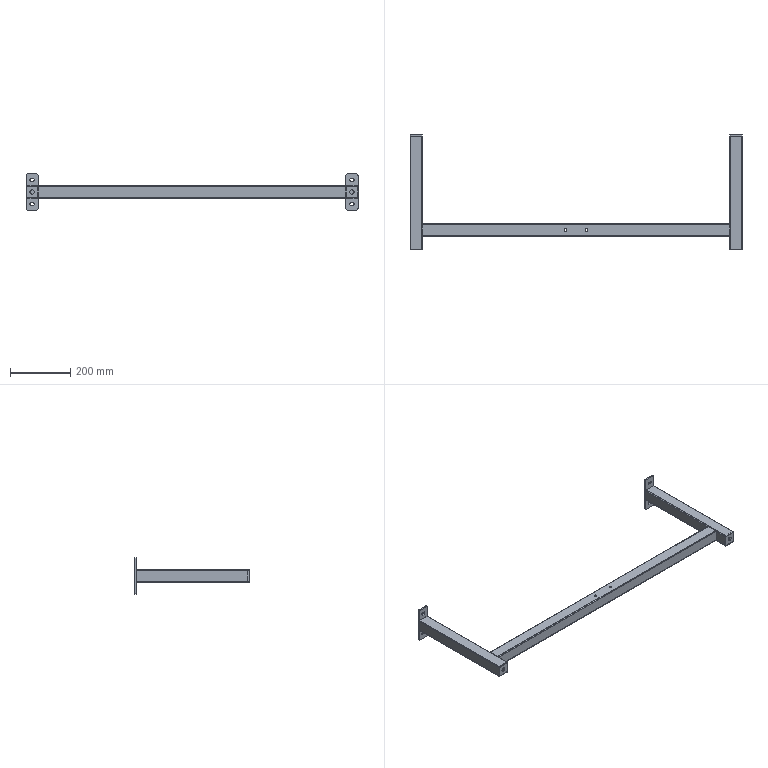Part | SolidWorks | features BaseBody 7 | 7 solids | 122 faces | box 1100 x 380 x 120 mm | volume 454651 mm3 | plane 62 | cylinder 60 | commonest cylinder face diameters 6 x20 9 x16 3 x12 10 x8 14 x4